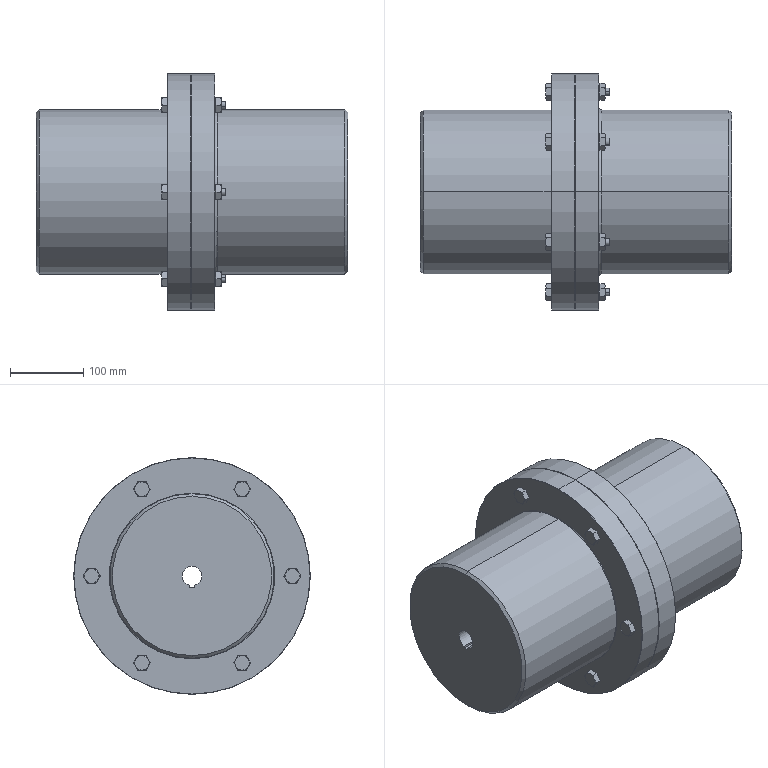Part | SolidWorks | features ICE 15, Chamfer 6, Revolution 3, CirPattern 2, Fillet 2, Scale 1 | 1 solid | 433 faces | box 423.5 x 322 x 322 mm | volume 19008725 mm3 | plane 223 | cone 144 | cylinder 62 | torus 4 | commonest cylinder face diameters 9.8 x36 19.6 x12 224 x7 322 x4 26.6 x3